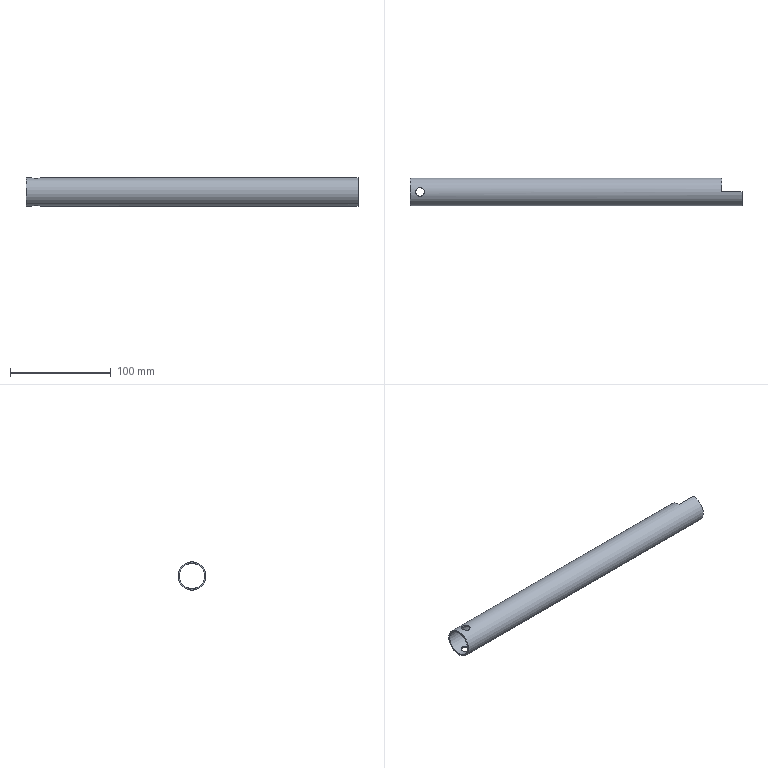Part | STEP file | GAS SHOCK 610W | 1 solid | 9 faces | box 330 x 28 x 28 mm | volume 39789 mm3 | plane 5 | cylinder 4 | commonest cylinder face diameters 8.5 x2 25 x1 28 x1